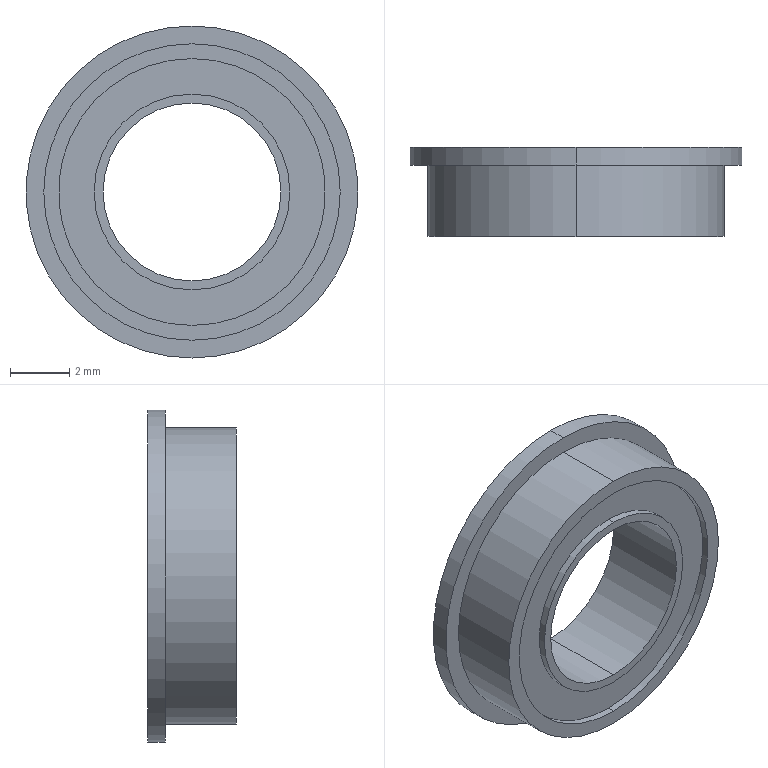Part | NX | features BREP 1 | 1 solid | 21 faces | box 11.2 x 3 x 11.2 mm | volume 148.082 mm3 | cylinder 14 | plane 7 | commonest cylinder face diameters 6.6 x4 9 x4 6 x2 10 x2 11.2 x2
STEP:
#1=CARTESIAN_POINT('',(0.,3.,-3.3));
#2=VERTEX_POINT('',#1);
#3=CARTESIAN_POINT('',(0.,2.75,-3.3));
#4=VERTEX_POINT('',#3);
#5=CARTESIAN_POINT('',(0.,2.75,-3.3));
#6=DIRECTION('',(0.,1.,0.));
#7=VECTOR('',#6,1000.);
#8=LINE('',#5,#7);
#9=EDGE_CURVE('',#2,#4,#8,.F.);
#10=ORIENTED_EDGE('',*,*,#9,.T.);
#11=CARTESIAN_POINT('',(0.,2.75,3.3));
#12=VERTEX_POINT('',#11);
#13=CARTESIAN_POINT('',(0.,2.75,0.));
#14=DIRECTION('',(0.,1.,0.));
#15=DIRECTION('',(0.,0.,1.));
#16=AXIS2_PLACEMENT_3D('',#13,#14,#15);
#17=CIRCLE('',#16,3.3);
#18=EDGE_CURVE('',#4,#12,#17,.T.);
#19=ORIENTED_EDGE('',*,*,#18,.T.);
#20=CARTESIAN_POINT('',(0.,3.,3.3));
#21=VERTEX_POINT('',#20);
#22=CARTESIAN_POINT('',(0.,2.75,3.3));
#23=DIRECTION('',(0.,1.,0.));
#24=VECTOR('',#23,1000.);
#25=LINE('',#22,#24);
#26=EDGE_CURVE('',#21,#12,#25,.F.);
#27=ORIENTED_EDGE('',*,*,#26,.F.);
#28=CARTESIAN_POINT('',(0.,3.,0.));
#29=DIRECTION('',(0.,1.,0.));
#30=DIRECTION('',(0.,0.,1.));
#31=AXIS2_PLACEMENT_3D('',#28,#29,#30);
#32=CIRCLE('',#31,3.3);
#33=EDGE_CURVE('',#2,#21,#32,.T.);
#34=ORIENTED_EDGE('',*,*,#33,.F.);
#35=EDGE_LOOP('',(#10,#19,#27,#34));
#36=FACE_BOUND('',#35,.T.);
#37=CARTESIAN_POINT('',(0.,2.75,0.));
#38=DIRECTION('',(0.,1.,0.));
#39=DIRECTION('',(0.,0.,1.));
#40=AXIS2_PLACEMENT_3D('',#37,#38,#39);
#41=CYLINDRICAL_SURFACE('',#40,3.3);
#42=ADVANCED_FACE('',(#36),#41,.T.);
#43=CARTESIAN_POINT('',(0.,2.75,4.5));
#44=VERTEX_POINT('',#43);
#45=CARTESIAN_POINT('',(0.,2.75,-4.5));
#46=VERTEX_POINT('',#45);
#47=CARTESIAN_POINT('',(0.,2.75,0.));
#48=DIRECTION('',(0.,1.,0.));
#49=DIRECTION('',(0.,0.,1.));
#50=AXIS2_PLACEMENT_3D('',#47,#48,#49);
#51=CIRCLE('',#50,4.5);
#52=EDGE_CURVE('',#44,#46,#51,.T.);
#53=ORIENTED_EDGE('',*,*,#52,.T.);
#54=CARTESIAN_POINT('',(0.,2.75,0.));
#55=DIRECTION('',(0.,1.,0.));
#56=DIRECTION('',(0.,0.,1.));
#57=AXIS2_PLACEMENT_3D('',#54,#55,#56);
#58=CIRCLE('',#57,4.5);
#59=EDGE_CURVE('',#46,#44,#58,.T.);
#60=ORIENTED_EDGE('',*,*,#59,.T.);
#61=EDGE_LOOP('',(#53,#60));
#62=FACE_BOUND('',#61,.T.);
#63=CARTESIAN_POINT('',(0.,2.75,0.));
#64=DIRECTION('',(0.,1.,0.));
#65=DIRECTION('',(0.,0.,1.));
#66=AXIS2_PLACEMENT_3D('',#63,#64,#65);
#67=CIRCLE('',#66,3.3);
#68=EDGE_CURVE('',#12,#4,#67,.T.);
#69=ORIENTED_EDGE('',*,*,#68,.F.);
#70=ORIENTED_EDGE('',*,*,#18,.F.);
#71=EDGE_LOOP('',(#69,#70));
#72=FACE_BOUND('',#71,.T.);
#73=CARTESIAN_POINT('',(0.,2.75,0.));
#74=DIRECTION('',(0.,1.,0.));
#75=DIRECTION('',(0.,0.,1.));
#76=AXIS2_PLACEMENT_3D('',#73,#74,#75);
#77=PLANE('',#76);
#78=ADVANCED_FACE('',(#62,#72),#77,.T.);
#79=CARTESIAN_POINT('',(0.,3.,-4.5));
#80=VERTEX_POINT('',#79);
#81=CARTESIAN_POINT('',(0.,2.75,-4.5));
#82=DIRECTION('',(0.,1.,0.));
#83=VECTOR('',#82,1000.);
#84=LINE('',#81,#83);
#85=EDGE_CURVE('',#80,#46,#84,.F.);
#86=ORIENTED_EDGE('',*,*,#85,.T.);
#87=ORIENTED_EDGE('',*,*,#52,.F.);
#88=CARTESIAN_POINT('',(0.,3.,4.5));
#89=VERTEX_POINT('',#88);
#90=CARTESIAN_POINT('',(0.,2.75,4.5));
#91=DIRECTION('',(0.,1.,0.));
#92=VECTOR('',#91,1000.);
#93=LINE('',#90,#92);
#94=EDGE_CURVE('',#89,#44,#93,.F.);
#95=ORIENTED_EDGE('',*,*,#94,.F.);
#96=CARTESIAN_POINT('',(0.,3.,0.));
#97=DIRECTION('',(0.,1.,0.));
#98=DIRECTION('',(0.,0.,1.));
#99=AXIS2_PLACEMENT_3D('',#96,#97,#98);
#100=CIRCLE('',#99,4.5);
#101=EDGE_CURVE('',#89,#80,#100,.T.);
#102=ORIENTED_EDGE('',*,*,#101,.T.);
#103=EDGE_LOOP('',(#86,#87,#95,#102));
#104=FACE_BOUND('',#103,.T.);
#105=CARTESIAN_POINT('',(0.,2.75,0.));
#106=DIRECTION('',(0.,1.,0.));
#107=DIRECTION('',(0.,0.,1.));
#108=AXIS2_PLACEMENT_3D('',#105,#106,#107);
#109=CYLINDRICAL_SURFACE('',#108,4.5);
#110=ADVANCED_FACE('',(#104),#109,.F.);
#111=CARTESIAN_POINT('',(0.,0.25,3.3));
#112=VERTEX_POINT('',#111);
#113=CARTESIAN_POINT('',(0.,0.,3.3));
#114=VERTEX_POINT('',#113);
#115=CARTESIAN_POINT('',(0.,0.25,3.3));
#116=DIRECTION('',(0.,-1.,0.));
#117=VECTOR('',#116,1000.);
#118=LINE('',#115,#117);
#119=EDGE_CURVE('',#112,#114,#118,.T.);
#120=ORIENTED_EDGE('',*,*,#119,.F.);
#121=CARTESIAN_POINT('',(0.,0.25,-3.3));
#122=VERTEX_POINT('',#121);
#123=CARTESIAN_POINT('',(0.,0.25,0.));
#124=DIRECTION('',(0.,-1.,0.));
#125=DIRECTION('',(0.,0.,-1.));
#126=AXIS2_PLACEMENT_3D('',#123,#124,#125);
#127=CIRCLE('',#126,3.3);
#128=EDGE_CURVE('',#112,#122,#127,.T.);
#129=ORIENTED_EDGE('',*,*,#128,.T.);
#130=CARTESIAN_POINT('',(0.,0.,-3.3));
#131=VERTEX_POINT('',#130);
#132=CARTESIAN_POINT('',(0.,0.25,-3.3));
#133=DIRECTION('',(0.,-1.,0.));
#134=VECTOR('',#133,1000.);
#135=LINE('',#132,#134);
#136=EDGE_CURVE('',#122,#131,#135,.T.);
#137=ORIENTED_EDGE('',*,*,#136,.T.);
#138=CARTESIAN_POINT('',(0.,0.,0.));
#139=DIRECTION('',(0.,-1.,0.));
#140=DIRECTION('',(0.,0.,-1.));
#141=AXIS2_PLACEMENT_3D('',#138,#139,#140);
#142=CIRCLE('',#141,3.3);
#143=EDGE_CURVE('',#114,#131,#142,.T.);
#144=ORIENTED_EDGE('',*,*,#143,.F.);
#145=EDGE_LOOP('',(#120,#129,#137,#144));
#146=FACE_BOUND('',#145,.T.);
#147=CARTESIAN_POINT('',(0.,0.25,0.));
#148=DIRECTION('',(0.,-1.,0.));
#149=DIRECTION('',(0.,0.,-1.));
#150=AXIS2_PLACEMENT_3D('',#147,#148,#149);
#151=CYLINDRICAL_SURFACE('',#150,3.3);
#152=ADVANCED_FACE('',(#146),#151,.T.);
#153=CARTESIAN_POINT('',(0.,0.25,-4.5));
#154=VERTEX_POINT('',#153);
#155=CARTESIAN_POINT('',(0.,0.25,4.5));
#156=VERTEX_POINT('',#155);
#157=CARTESIAN_POINT('',(0.,0.25,0.));
#158=DIRECTION('',(0.,-1.,0.));
#159=DIRECTION('',(0.,0.,-1.));
#160=AXIS2_PLACEMENT_3D('',#157,#158,#159);
#161=CIRCLE('',#160,4.5);
#162=EDGE_CURVE('',#154,#156,#161,.T.);
#163=ORIENTED_EDGE('',*,*,#162,.T.);
#164=CARTESIAN_POINT('',(0.,0.25,0.));
#165=DIRECTION('',(0.,-1.,0.));
#166=DIRECTION('',(0.,0.,-1.));
#167=AXIS2_PLACEMENT_3D('',#164,#165,#166);
#168=CIRCLE('',#167,4.5);
#169=EDGE_CURVE('',#156,#154,#168,.T.);
#170=ORIENTED_EDGE('',*,*,#169,.T.);
#171=EDGE_LOOP('',(#163,#170));
#172=FACE_BOUND('',#171,.T.);
#173=CARTESIAN_POINT('',(0.,0.25,0.));
#174=DIRECTION('',(0.,-1.,0.));
#175=DIRECTION('',(0.,0.,-1.));
#176=AXIS2_PLACEMENT_3D('',#173,#174,#175);
#177=CIRCLE('',#176,3.3);
#178=EDGE_CURVE('',#122,#112,#177,.T.);
#179=ORIENTED_EDGE('',*,*,#178,.F.);
#180=ORIENTED_EDGE('',*,*,#128,.F.);
#181=EDGE_LOOP('',(#179,#180));
#182=FACE_BOUND('',#181,.T.);
#183=CARTESIAN_POINT('',(0.,0.25,0.));
#184=DIRECTION('',(0.,-1.,0.));
#185=DIRECTION('',(0.,0.,-1.));
#186=AXIS2_PLACEMENT_3D('',#183,#184,#185);
#187=PLANE('',#186);
#188=ADVANCED_FACE('',(#172,#182),#187,.T.);
#189=CARTESIAN_POINT('',(0.,0.,4.5));
#190=VERTEX_POINT('',#189);
#191=CARTESIAN_POINT('',(0.,0.25,4.5));
#192=DIRECTION('',(0.,-1.,0.));
#193=VECTOR('',#192,1000.);
#194=LINE('',#191,#193);
#195=EDGE_CURVE('',#156,#190,#194,.T.);
#196=ORIENTED_EDGE('',*,*,#195,.F.);
#197=ORIENTED_EDGE('',*,*,#162,.F.);
#198=CARTESIAN_POINT('',(0.,0.,-4.5));
#199=VERTEX_POINT('',#198);
#200=CARTESIAN_POINT('',(0.,0.25,-4.5));
#201=DIRECTION('',(0.,-1.,0.));
#202=VECTOR('',#201,1000.);
#203=LINE('',#200,#202);
#204=EDGE_CURVE('',#154,#199,#203,.T.);
#205=ORIENTED_EDGE('',*,*,#204,.T.);
#206=CARTESIAN_POINT('',(0.,0.,0.));
#207=DIRECTION('',(0.,-1.,0.));
#208=DIRECTION('',(0.,0.,-1.));
#209=AXIS2_PLACEMENT_3D('',#206,#207,#208);
#210=CIRCLE('',#209,4.5);
#211=EDGE_CURVE('',#199,#190,#210,.T.);
#212=ORIENTED_EDGE('',*,*,#211,.T.);
#213=EDGE_LOOP('',(#196,#197,#205,#212));
#214=FACE_BOUND('',#213,.T.);
#215=CARTESIAN_POINT('',(0.,0.25,0.));
#216=DIRECTION('',(0.,-1.,0.));
#217=DIRECTION('',(0.,0.,-1.));
#218=AXIS2_PLACEMENT_3D('',#215,#216,#217);
#219=CYLINDRICAL_SURFACE('',#218,4.5);
#220=ADVANCED_FACE('',(#214),#219,.F.);
#221=CARTESIAN_POINT('',(0.,2.4,5.));
#222=VERTEX_POINT('',#221);
#223=CARTESIAN_POINT('',(0.,0.,5.));
#224=VERTEX_POINT('',#223);
#225=CARTESIAN_POINT('',(0.,0.,5.));
#226=DIRECTION('',(0.,-1.,0.));
#227=VECTOR('',#226,1000.);
#228=LINE('',#225,#227);
#229=EDGE_CURVE('',#222,#224,#228,.T.);
#230=ORIENTED_EDGE('',*,*,#229,.F.);
#231=CARTESIAN_POINT('',(0.,2.4,-5.));
#232=VERTEX_POINT('',#231);
#233=CARTESIAN_POINT('',(0.,2.4,0.));
#234=DIRECTION('',(0.,-1.,0.));
#235=DIRECTION('',(0.,0.,-1.));
#236=AXIS2_PLACEMENT_3D('',#233,#234,#235);
#237=CIRCLE('',#236,5.);
#238=EDGE_CURVE('',#222,#232,#237,.T.);
#239=ORIENTED_EDGE('',*,*,#238,.T.);
#240=CARTESIAN_POINT('',(0.,0.,-5.));
#241=VERTEX_POINT('',#240);
#242=CARTESIAN_POINT('',(0.,0.,-5.));
#243=DIRECTION('',(0.,-1.,0.));
#244=VECTOR('',#243,1000.);
#245=LINE('',#242,#244);
#246=EDGE_CURVE('',#232,#241,#245,.T.);
#247=ORIENTED_EDGE('',*,*,#246,.T.);
#248=CARTESIAN_POINT('',(0.,0.,0.));
#249=DIRECTION('',(0.,-1.,0.));
#250=DIRECTION('',(0.,0.,-1.));
#251=AXIS2_PLACEMENT_3D('',#248,#249,#250);
#252=CIRCLE('',#251,5.);
#253=EDGE_CURVE('',#224,#241,#252,.T.);
#254=ORIENTED_EDGE('',*,*,#253,.F.);
#255=EDGE_LOOP('',(#230,#239,#247,#254));
#256=FACE_BOUND('',#255,.T.);
#257=CARTESIAN_POINT('',(0.,0.,0.));
#258=DIRECTION('',(0.,-1.,0.));
#259=DIRECTION('',(0.,0.,-1.));
#260=AXIS2_PLACEMENT_3D('',#257,#258,#259);
#261=CYLINDRICAL_SURFACE('',#260,5.);
#262=ADVANCED_FACE('',(#256),#261,.T.);
#263=CARTESIAN_POINT('',(0.,2.4,-5.6));
#264=VERTEX_POINT('',#263);
#265=CARTESIAN_POINT('',(0.,2.4,5.6));
#266=VERTEX_POINT('',#265);
#267=CARTESIAN_POINT('',(0.,2.4,0.));
#268=DIRECTION('',(0.,-1.,0.));
#269=DIRECTION('',(0.,0.,-1.));
#270=AXIS2_PLACEMENT_3D('',#267,#268,#269);
#271=CIRCLE('',#270,5.6);
#272=EDGE_CURVE('',#264,#266,#271,.T.);
#273=ORIENTED_EDGE('',*,*,#272,.T.);
#274=CARTESIAN_POINT('',(0.,2.4,0.));
#275=DIRECTION('',(0.,-1.,0.));
#276=DIRECTION('',(0.,0.,-1.));
#277=AXIS2_PLACEMENT_3D('',#274,#275,#276);
#278=CIRCLE('',#277,5.6);
#279=EDGE_CURVE('',#266,#264,#278,.T.);
#280=ORIENTED_EDGE('',*,*,#279,.T.);
#281=EDGE_LOOP('',(#273,#280));
#282=FACE_BOUND('',#281,.T.);
#283=CARTESIAN_POINT('',(0.,2.4,0.));
#284=DIRECTION('',(0.,-1.,0.));
#285=DIRECTION('',(0.,0.,-1.));
#286=AXIS2_PLACEMENT_3D('',#283,#284,#285);
#287=CIRCLE('',#286,5.);
#288=EDGE_CURVE('',#232,#222,#287,.T.);
#289=ORIENTED_EDGE('',*,*,#288,.F.);
#290=ORIENTED_EDGE('',*,*,#238,.F.);
#291=EDGE_LOOP('',(#289,#290));
#292=FACE_BOUND('',#291,.T.);
#293=CARTESIAN_POINT('',(-5.6,2.4,0.));
#294=DIRECTION('',(0.,1.,0.));
#295=DIRECTION('',(0.,0.,1.));
#296=AXIS2_PLACEMENT_3D('',#293,#294,#295);
#297=PLANE('',#296);
#298=ADVANCED_FACE('',(#282,#292),#297,.F.);
#299=CARTESIAN_POINT('',(0.,3.,5.6));
#300=VERTEX_POINT('',#299);
#301=CARTESIAN_POINT('',(0.,0.,5.6));
#302=DIRECTION('',(0.,-1.,0.));
#303=VECTOR('',#302,1000.);
#304=LINE('',#301,#303);
#305=EDGE_CURVE('',#300,#266,#304,.T.);
#306=ORIENTED_EDGE('',*,*,#305,.F.);
#307=CARTESIAN_POINT('',(0.,3.,-5.6));
#308=VERTEX_POINT('',#307);
#309=CARTESIAN_POINT('',(0.,3.,0.));
#310=DIRECTION('',(0.,-1.,0.));
#311=DIRECTION('',(0.,0.,-1.));
#312=AXIS2_PLACEMENT_3D('',#309,#310,#311);
#313=CIRCLE('',#312,5.6);
#314=EDGE_CURVE('',#300,#308,#313,.T.);
#315=ORIENTED_EDGE('',*,*,#314,.T.);
#316=CARTESIAN_POINT('',(0.,0.,-5.6));
#317=DIRECTION('',(0.,-1.,0.));
#318=VECTOR('',#317,1000.);
#319=LINE('',#316,#318);
#320=EDGE_CURVE('',#308,#264,#319,.T.);
#321=ORIENTED_EDGE('',*,*,#320,.T.);
#322=ORIENTED_EDGE('',*,*,#279,.F.);
#323=EDGE_LOOP('',(#306,#315,#321,#322));
#324=FACE_BOUND('',#323,.T.);
#325=CARTESIAN_POINT('',(0.,0.,0.));
#326=DIRECTION('',(0.,-1.,0.));
#327=DIRECTION('',(0.,0.,-1.));
#328=AXIS2_PLACEMENT_3D('',#325,#326,#327);
#329=CYLINDRICAL_SURFACE('',#328,5.6);
#330=ADVANCED_FACE('',(#324),#329,.T.);
#331=CARTESIAN_POINT('',(0.,3.,0.));
#332=DIRECTION('',(0.,-1.,0.));
#333=DIRECTION('',(0.,0.,-1.));
#334=AXIS2_PLACEMENT_3D('',#331,#332,#333);
#335=CIRCLE('',#334,5.6);
#336=EDGE_CURVE('',#308,#300,#335,.T.);
#337=ORIENTED_EDGE('',*,*,#336,.F.);
#338=ORIENTED_EDGE('',*,*,#314,.F.);
#339=EDGE_LOOP('',(#337,#338));
#340=FACE_BOUND('',#339,.T.);
#341=ORIENTED_EDGE('',*,*,#101,.F.);
#342=CARTESIAN_POINT('',(0.,3.,0.));
#343=DIRECTION('',(0.,1.,0.));
#344=DIRECTION('',(0.,0.,1.));
#345=AXIS2_PLACEMENT_3D('',#342,#343,#344);
#346=CIRCLE('',#345,4.5);
#347=EDGE_CURVE('',#80,#89,#346,.T.);
#348=ORIENTED_EDGE('',*,*,#347,.F.);
#349=EDGE_LOOP('',(#341,#348));
#350=FACE_BOUND('',#349,.T.);
#351=CARTESIAN_POINT('',(-3.,3.,0.));
#352=DIRECTION('',(0.,-1.,0.));
#353=DIRECTION('',(0.,0.,-1.));
#354=AXIS2_PLACEMENT_3D('',#351,#352,#353);
#355=PLANE('',#354);
#356=ADVANCED_FACE('',(#340,#350),#355,.F.);
#357=CARTESIAN_POINT('',(0.,3.,3.));
#358=VERTEX_POINT('',#357);
#359=CARTESIAN_POINT('',(0.,0.,3.));
#360=VERTEX_POINT('',#359);
#361=CARTESIAN_POINT('',(0.,0.,3.));
#362=DIRECTION('',(0.,-1.,0.));
#363=VECTOR('',#362,1000.);
#364=LINE('',#361,#363);
#365=EDGE_CURVE('',#358,#360,#364,.T.);
#366=ORIENTED_EDGE('',*,*,#365,.F.);
#367=CARTESIAN_POINT('',(0.,3.,-3.));
#368=VERTEX_POINT('',#367);
#369=CARTESIAN_POINT('',(0.,3.,0.));
#370=DIRECTION('',(0.,-1.,0.));
#371=DIRECTION('',(0.,0.,-1.));
#372=AXIS2_PLACEMENT_3D('',#369,#370,#371);
#373=CIRCLE('',#372,3.);
#374=EDGE_CURVE('',#368,#358,#373,.T.);
#375=ORIENTED_EDGE('',*,*,#374,.F.);
#376=CARTESIAN_POINT('',(0.,0.,-3.));
#377=VERTEX_POINT('',#376);
#378=CARTESIAN_POINT('',(0.,0.,-3.));
#379=DIRECTION('',(0.,-1.,0.));
#380=VECTOR('',#379,1000.);
#381=LINE('',#378,#380);
#382=EDGE_CURVE('',#368,#377,#381,.T.);
#383=ORIENTED_EDGE('',*,*,#382,.T.);
#384=CARTESIAN_POINT('',(0.,0.,0.));
#385=DIRECTION('',(0.,-1.,0.));
#386=DIRECTION('',(0.,0.,-1.));
#387=AXIS2_PLACEMENT_3D('',#384,#385,#386);
#388=CIRCLE('',#387,3.);
#389=EDGE_CURVE('',#377,#360,#388,.T.);
#390=ORIENTED_EDGE('',*,*,#389,.T.);
#391=EDGE_LOOP('',(#366,#375,#383,#390));
#392=FACE_BOUND('',#391,.T.);
#393=CARTESIAN_POINT('',(0.,0.,0.));
#394=DIRECTION('',(0.,-1.,0.));
#395=DIRECTION('',(0.,0.,-1.));
#396=AXIS2_PLACEMENT_3D('',#393,#394,#395);
#397=CYLINDRICAL_SURFACE('',#396,3.);
#398=ADVANCED_FACE('',(#392),#397,.F.);
#399=CARTESIAN_POINT('',(0.,0.,0.));
#400=DIRECTION('',(0.,-1.,0.));
#401=DIRECTION('',(0.,0.,-1.));
#402=AXIS2_PLACEMENT_3D('',#399,#400,#401);
#403=CIRCLE('',#402,5.);
#404=EDGE_CURVE('',#241,#224,#403,.T.);
#405=ORIENTED_EDGE('',*,*,#404,.T.);
#406=ORIENTED_EDGE('',*,*,#253,.T.);
#407=EDGE_LOOP('',(#405,#406));
#408=FACE_BOUND('',#407,.T.);
#409=ORIENTED_EDGE('',*,*,#211,.F.);
#410=CARTESIAN_POINT('',(0.,0.,0.));
#411=DIRECTION('',(0.,-1.,0.));
#412=DIRECTION('',(0.,0.,-1.));
#413=AXIS2_PLACEMENT_3D('',#410,#411,#412);
#414=CIRCLE('',#413,4.5);
#415=EDGE_CURVE('',#190,#199,#414,.T.);
#416=ORIENTED_EDGE('',*,*,#415,.F.);
#417=EDGE_LOOP('',(#409,#416));
#418=FACE_BOUND('',#417,.T.);
#419=CARTESIAN_POINT('',(-5.,0.,0.));
#420=DIRECTION('',(0.,1.,0.));
#421=DIRECTION('',(0.,0.,1.));
#422=AXIS2_PLACEMENT_3D('',#419,#420,#421);
#423=PLANE('',#422);
#424=ADVANCED_FACE('',(#408,#418),#423,.F.);
#425=CARTESIAN_POINT('',(0.,0.,0.));
#426=DIRECTION('',(0.,-1.,0.));
#427=DIRECTION('',(0.,0.,-1.));
#428=AXIS2_PLACEMENT_3D('',#425,#426,#427);
#429=CIRCLE('',#428,3.3);
#430=EDGE_CURVE('',#131,#114,#429,.T.);
#431=ORIENTED_EDGE('',*,*,#430,.T.);
#432=ORIENTED_EDGE('',*,*,#143,.T.);
#433=EDGE_LOOP('',(#431,#432));
#434=FACE_BOUND('',#433,.T.);
#435=ORIENTED_EDGE('',*,*,#389,.F.);
#436=CARTESIAN_POINT('',(0.,0.,0.));
#437=DIRECTION('',(0.,-1.,0.));
#438=DIRECTION('',(0.,0.,-1.));
#439=AXIS2_PLACEMENT_3D('',#436,#437,#438);
#440=CIRCLE('',#439,3.);
#441=EDGE_CURVE('',#360,#377,#440,.T.);
#442=ORIENTED_EDGE('',*,*,#441,.F.);
#443=EDGE_LOOP('',(#435,#442));
#444=FACE_BOUND('',#443,.T.);
#445=CARTESIAN_POINT('',(-5.,0.,0.));
#446=DIRECTION('',(0.,1.,0.));
#447=DIRECTION('',(0.,0.,1.));
#448=AXIS2_PLACEMENT_3D('',#445,#446,#447);
#449=PLANE('',#448);
#450=ADVANCED_FACE('',(#434,#444),#449,.F.);
#451=CARTESIAN_POINT('',(0.,3.,0.));
#452=DIRECTION('',(0.,1.,0.));
#453=DIRECTION('',(0.,0.,1.));
#454=AXIS2_PLACEMENT_3D('',#451,#452,#453);
#455=CIRCLE('',#454,3.3);
#456=EDGE_CURVE('',#21,#2,#455,.T.);
#457=ORIENTED_EDGE('',*,*,#456,.T.);
#458=ORIENTED_EDGE('',*,*,#33,.T.);
#459=EDGE_LOOP('',(#457,#458));
#460=FACE_BOUND('',#459,.T.);
#461=ORIENTED_EDGE('',*,*,#374,.T.);
#462=CARTESIAN_POINT('',(0.,3.,0.));
#463=DIRECTION('',(0.,-1.,0.));
#464=DIRECTION('',(0.,0.,-1.));
#465=AXIS2_PLACEMENT_3D('',#462,#463,#464);
#466=CIRCLE('',#465,3.);
#467=EDGE_CURVE('',#358,#368,#466,.T.);
#468=ORIENTED_EDGE('',*,*,#467,.T.);
#469=EDGE_LOOP('',(#461,#468));
#470=FACE_BOUND('',#469,.T.);
#471=CARTESIAN_POINT('',(-3.,3.,0.));
#472=DIRECTION('',(0.,-1.,0.));
#473=DIRECTION('',(0.,0.,-1.));
#474=AXIS2_PLACEMENT_3D('',#471,#472,#473);
#475=PLANE('',#474);
#476=ADVANCED_FACE('',(#460,#470),#475,.F.);
#477=ORIENTED_EDGE('',*,*,#467,.F.);
#478=ORIENTED_EDGE('',*,*,#365,.T.);
#479=ORIENTED_EDGE('',*,*,#441,.T.);
#480=ORIENTED_EDGE('',*,*,#382,.F.);
#481=EDGE_LOOP('',(#477,#478,#479,#480));
#482=FACE_BOUND('',#481,.T.);
#483=CARTESIAN_POINT('',(0.,0.,0.));
#484=DIRECTION('',(0.,-1.,0.));
#485=DIRECTION('',(0.,0.,-1.));
#486=AXIS2_PLACEMENT_3D('',#483,#484,#485);
#487=CYLINDRICAL_SURFACE('',#486,3.);
#488=ADVANCED_FACE('',(#482),#487,.F.);
#489=ORIENTED_EDGE('',*,*,#336,.T.);
#490=ORIENTED_EDGE('',*,*,#305,.T.);
#491=ORIENTED_EDGE('',*,*,#272,.F.);
#492=ORIENTED_EDGE('',*,*,#320,.F.);
#493=EDGE_LOOP('',(#489,#490,#491,#492));
#494=FACE_BOUND('',#493,.T.);
#495=CARTESIAN_POINT('',(0.,0.,0.));
#496=DIRECTION('',(0.,-1.,0.));
#497=DIRECTION('',(0.,0.,-1.));
#498=AXIS2_PLACEMENT_3D('',#495,#496,#497);
#499=CYLINDRICAL_SURFACE('',#498,5.6);
#500=ADVANCED_FACE('',(#494),#499,.T.);
#501=ORIENTED_EDGE('',*,*,#288,.T.);
#502=ORIENTED_EDGE('',*,*,#229,.T.);
#503=ORIENTED_EDGE('',*,*,#404,.F.);
#504=ORIENTED_EDGE('',*,*,#246,.F.);
#505=EDGE_LOOP('',(#501,#502,#503,#504));
#506=FACE_BOUND('',#505,.T.);
#507=CARTESIAN_POINT('',(0.,0.,0.));
#508=DIRECTION('',(0.,-1.,0.));
#509=DIRECTION('',(0.,0.,-1.));
#510=AXIS2_PLACEMENT_3D('',#507,#508,#509);
#511=CYLINDRICAL_SURFACE('',#510,5.);
#512=ADVANCED_FACE('',(#506),#511,.T.);
#513=ORIENTED_EDGE('',*,*,#169,.F.);
#514=ORIENTED_EDGE('',*,*,#195,.T.);
#515=ORIENTED_EDGE('',*,*,#415,.T.);
#516=ORIENTED_EDGE('',*,*,#204,.F.);
#517=EDGE_LOOP('',(#513,#514,#515,#516));
#518=FACE_BOUND('',#517,.T.);
#519=CARTESIAN_POINT('',(0.,0.25,0.));
#520=DIRECTION('',(0.,-1.,0.));
#521=DIRECTION('',(0.,0.,-1.));
#522=AXIS2_PLACEMENT_3D('',#519,#520,#521);
#523=CYLINDRICAL_SURFACE('',#522,4.5);
#524=ADVANCED_FACE('',(#518),#523,.F.);
#525=ORIENTED_EDGE('',*,*,#178,.T.);
#526=ORIENTED_EDGE('',*,*,#119,.T.);
#527=ORIENTED_EDGE('',*,*,#430,.F.);
#528=ORIENTED_EDGE('',*,*,#136,.F.);
#529=EDGE_LOOP('',(#525,#526,#527,#528));
#530=FACE_BOUND('',#529,.T.);
#531=CARTESIAN_POINT('',(0.,0.25,0.));
#532=DIRECTION('',(0.,-1.,0.));
#533=DIRECTION('',(0.,0.,-1.));
#534=AXIS2_PLACEMENT_3D('',#531,#532,#533);
#535=CYLINDRICAL_SURFACE('',#534,3.3);
#536=ADVANCED_FACE('',(#530),#535,.T.);
#537=ORIENTED_EDGE('',*,*,#59,.F.);
#538=ORIENTED_EDGE('',*,*,#85,.F.);
#539=ORIENTED_EDGE('',*,*,#347,.T.);
#540=ORIENTED_EDGE('',*,*,#94,.T.);
#541=EDGE_LOOP('',(#537,#538,#539,#540));
#542=FACE_BOUND('',#541,.T.);
#543=CARTESIAN_POINT('',(0.,2.75,0.));
#544=DIRECTION('',(0.,1.,0.));
#545=DIRECTION('',(0.,0.,1.));
#546=AXIS2_PLACEMENT_3D('',#543,#544,#545);
#547=CYLINDRICAL_SURFACE('',#546,4.5);
#548=ADVANCED_FACE('',(#542),#547,.F.);
#549=ORIENTED_EDGE('',*,*,#68,.T.);
#550=ORIENTED_EDGE('',*,*,#9,.F.);
#551=ORIENTED_EDGE('',*,*,#456,.F.);
#552=ORIENTED_EDGE('',*,*,#26,.T.);
#553=EDGE_LOOP('',(#549,#550,#551,#552));
#554=FACE_BOUND('',#553,.T.);
#555=CARTESIAN_POINT('',(0.,2.75,0.));
#556=DIRECTION('',(0.,1.,0.));
#557=DIRECTION('',(0.,0.,1.));
#558=AXIS2_PLACEMENT_3D('',#555,#556,#557);
#559=CYLINDRICAL_SURFACE('',#558,3.3);
#560=ADVANCED_FACE('',(#554),#559,.T.);
#561=CLOSED_SHELL('',(#42,#78,#110,#152,#188,#220,#262,#298,#330,#356,#398,#424,#450,#476,#488,#500,#512,#524,#536,#548,#560));
#562=MANIFOLD_SOLID_BREP('',#561);
#563=(LENGTH_UNIT()NAMED_UNIT(*)SI_UNIT(.MILLI.,.METRE.));
#564=UNCERTAINTY_MEASURE_WITH_UNIT(LENGTH_MEASURE(0.00001),#563,'','');
#565=(NAMED_UNIT(*)PLANE_ANGLE_UNIT()SI_UNIT($,.RADIAN.));
#566=(NAMED_UNIT(*)SI_UNIT($,.STERADIAN.)SOLID_ANGLE_UNIT());
#567=(GEOMETRIC_REPRESENTATION_CONTEXT(3)GLOBAL_UNCERTAINTY_ASSIGNED_CONTEXT((#564))GLOBAL_UNIT_ASSIGNED_CONTEXT((#563,#565,#566))REPRESENTATION_CONTEXT('',''));
#568=ADVANCED_BREP_SHAPE_REPRESENTATION('',(#562),#567);